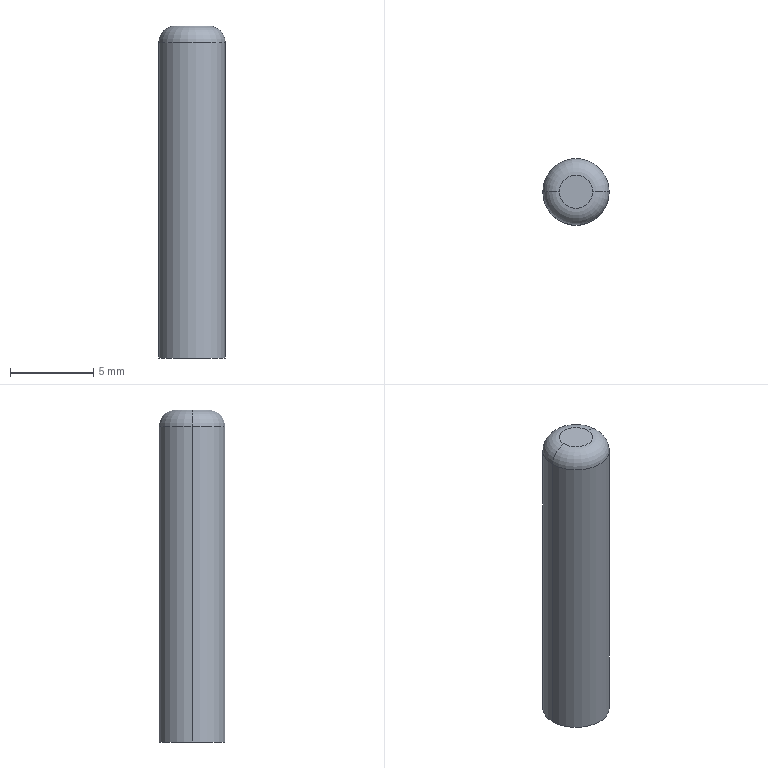Part | SolidWorks | features MirrorStock 1 | 1 solid | 10 faces | box 4 x 4 x 20 mm | volume 245.594 mm3 | cylinder 4 | torus 2 | cone 2 | plane 2 | commonest cylinder face diameters 1.6 x2 4 x2
STEP:
#1=CARTESIAN_POINT('',(11.281,-38.2,0.));
#2=VERTEX_POINT('',#1);
#3=CARTESIAN_POINT('',(9.281,-38.2,0.));
#4=VERTEX_POINT('',#3);
#5=CARTESIAN_POINT('',(10.281,-38.2,0.));
#6=DIRECTION('',(0.,0.,-1.));
#7=DIRECTION('',(1.,0.,0.));
#8=AXIS2_PLACEMENT_3D('',#5,#6,#7);
#9=CIRCLE('',#8,1.);
#10=EDGE_CURVE('',#2,#4,#9,.T.);
#11=ORIENTED_EDGE('',*,*,#10,.T.);
#12=CARTESIAN_POINT('',(8.281,-38.2,-1.));
#13=VERTEX_POINT('',#12);
#14=CARTESIAN_POINT('',(9.281,-38.2,-1.));
#15=DIRECTION('',(0.,-1.,0.));
#16=DIRECTION('',(1.,0.,0.));
#17=AXIS2_PLACEMENT_3D('',#14,#15,#16);
#18=CIRCLE('',#17,1.);
#19=EDGE_CURVE('',#4,#13,#18,.T.);
#20=ORIENTED_EDGE('',*,*,#19,.T.);
#21=CARTESIAN_POINT('',(12.281,-38.2,-1.));
#22=VERTEX_POINT('',#21);
#23=CARTESIAN_POINT('',(10.281,-38.2,-1.));
#24=DIRECTION('',(0.,0.,1.));
#25=DIRECTION('',(1.,0.,0.));
#26=AXIS2_PLACEMENT_3D('',#23,#24,#25);
#27=CIRCLE('',#26,2.);
#28=EDGE_CURVE('',#13,#22,#27,.T.);
#29=ORIENTED_EDGE('',*,*,#28,.T.);
#30=CARTESIAN_POINT('',(11.281,-38.2,-1.));
#31=DIRECTION('',(0.,1.,0.));
#32=DIRECTION('',(0.,0.,1.));
#33=AXIS2_PLACEMENT_3D('',#30,#31,#32);
#34=CIRCLE('',#33,1.);
#35=EDGE_CURVE('',#2,#22,#34,.T.);
#36=ORIENTED_EDGE('',*,*,#35,.F.);
#37=EDGE_LOOP('',(#11,#20,#29,#36));
#38=FACE_OUTER_BOUND('',#37,.T.);
#39=CARTESIAN_POINT('',(10.281,-38.2,-1.));
#40=DIRECTION('',(0.,0.,-1.));
#41=DIRECTION('',(1.,0.,0.));
#42=AXIS2_PLACEMENT_3D('',#39,#40,#41);
#43=TOROIDAL_SURFACE('',#42,1.,1.);
#44=ADVANCED_FACE('',(#38),#43,.T.);
#45=CARTESIAN_POINT('',(10.281,-39.,-18.5));
#46=VERTEX_POINT('',#45);
#47=CARTESIAN_POINT('',(10.281,-37.4,-18.5));
#48=VERTEX_POINT('',#47);
#49=CARTESIAN_POINT('',(10.281,-38.2,-18.5));
#50=DIRECTION('',(0.,0.,1.));
#51=DIRECTION('',(0.,-1.,0.));
#52=AXIS2_PLACEMENT_3D('',#49,#50,#51);
#53=CIRCLE('',#52,0.8);
#54=EDGE_CURVE('',#46,#48,#53,.T.);
#55=ORIENTED_EDGE('',*,*,#54,.T.);
#56=CARTESIAN_POINT('',(10.281,-37.4,-20.));
#57=VERTEX_POINT('',#56);
#58=CARTESIAN_POINT('',(10.281,-37.4,-23.7));
#59=DIRECTION('',(0.,0.,-1.));
#60=VECTOR('',#59,1000.);
#61=LINE('',#58,#60);
#62=EDGE_CURVE('',#48,#57,#61,.T.);
#63=ORIENTED_EDGE('',*,*,#62,.T.);
#64=CARTESIAN_POINT('',(10.281,-39.,-20.));
#65=VERTEX_POINT('',#64);
#66=CARTESIAN_POINT('',(10.281,-38.2,-20.));
#67=DIRECTION('',(0.,0.,1.));
#68=DIRECTION('',(1.,0.,0.));
#69=AXIS2_PLACEMENT_3D('',#66,#67,#68);
#70=CIRCLE('',#69,0.8);
#71=EDGE_CURVE('',#65,#57,#70,.T.);
#72=ORIENTED_EDGE('',*,*,#71,.F.);
#73=CARTESIAN_POINT('',(10.281,-39.,-23.7));
#74=DIRECTION('',(0.,0.,-1.));
#75=VECTOR('',#74,1000.);
#76=LINE('',#73,#75);
#77=EDGE_CURVE('',#46,#65,#76,.T.);
#78=ORIENTED_EDGE('',*,*,#77,.F.);
#79=EDGE_LOOP('',(#55,#63,#72,#78));
#80=FACE_OUTER_BOUND('',#79,.T.);
#81=CARTESIAN_POINT('',(10.281,-38.2,-23.7));
#82=DIRECTION('',(0.,0.,-1.));
#83=DIRECTION('',(0.,-1.,0.));
#84=AXIS2_PLACEMENT_3D('',#81,#82,#83);
#85=CYLINDRICAL_SURFACE('',#84,0.8);
#86=ADVANCED_FACE('',(#80),#85,.F.);
#87=CARTESIAN_POINT('',(10.281,-38.2,-18.019));
#88=VERTEX_POINT('',#87);
#89=CARTESIAN_POINT('',(10.281,-39.,-18.5));
#90=DIRECTION('',(0.,-0.8572,-0.515));
#91=VECTOR('',#90,1000.);
#92=LINE('',#89,#91);
#93=EDGE_CURVE('',#88,#46,#92,.T.);
#94=ORIENTED_EDGE('',*,*,#93,.F.);
#95=CARTESIAN_POINT('',(10.281,-37.4,-18.5));
#96=DIRECTION('',(0.,0.8572,-0.515));
#97=VECTOR('',#96,1000.);
#98=LINE('',#95,#97);
#99=EDGE_CURVE('',#88,#48,#98,.T.);
#100=ORIENTED_EDGE('',*,*,#99,.T.);
#101=ORIENTED_EDGE('',*,*,#54,.F.);
#102=EDGE_LOOP('',(#94,#100,#101));
#103=FACE_OUTER_BOUND('',#102,.T.);
#104=CARTESIAN_POINT('',(10.281,-38.2,-18.5));
#105=DIRECTION('',(0.,0.,-1.));
#106=DIRECTION('',(0.,-1.,0.));
#107=AXIS2_PLACEMENT_3D('',#104,#105,#106);
#108=CONICAL_SURFACE('',#107,0.8,1.03);
#109=ADVANCED_FACE('',(#103),#108,.F.);
#110=CARTESIAN_POINT('',(8.281,-38.2,-20.));
#111=VERTEX_POINT('',#110);
#112=CARTESIAN_POINT('',(12.281,-38.2,-20.));
#113=VERTEX_POINT('',#112);
#114=CARTESIAN_POINT('',(10.281,-38.2,-20.));
#115=DIRECTION('',(0.,0.,1.));
#116=DIRECTION('',(1.,0.,0.));
#117=AXIS2_PLACEMENT_3D('',#114,#115,#116);
#118=CIRCLE('',#117,2.);
#119=EDGE_CURVE('',#111,#113,#118,.T.);
#120=ORIENTED_EDGE('',*,*,#119,.T.);
#121=CARTESIAN_POINT('',(12.281,-38.2,-20.));
#122=DIRECTION('',(0.,0.,1.));
#123=VECTOR('',#122,1000.);
#124=LINE('',#121,#123);
#125=EDGE_CURVE('',#113,#22,#124,.T.);
#126=ORIENTED_EDGE('',*,*,#125,.T.);
#127=ORIENTED_EDGE('',*,*,#28,.F.);
#128=CARTESIAN_POINT('',(8.281,-38.2,-20.));
#129=DIRECTION('',(0.,0.,1.));
#130=VECTOR('',#129,1000.);
#131=LINE('',#128,#130);
#132=EDGE_CURVE('',#111,#13,#131,.T.);
#133=ORIENTED_EDGE('',*,*,#132,.F.);
#134=EDGE_LOOP('',(#120,#126,#127,#133));
#135=FACE_OUTER_BOUND('',#134,.T.);
#136=CARTESIAN_POINT('',(10.281,-38.2,-20.));
#137=DIRECTION('',(0.,0.,1.));
#138=DIRECTION('',(-1.,0.,0.));
#139=AXIS2_PLACEMENT_3D('',#136,#137,#138);
#140=CYLINDRICAL_SURFACE('',#139,2.);
#141=ADVANCED_FACE('',(#135),#140,.T.);
#142=ORIENTED_EDGE('',*,*,#125,.F.);
#143=CARTESIAN_POINT('',(10.281,-38.2,-20.));
#144=DIRECTION('',(0.,0.,1.));
#145=DIRECTION('',(1.,0.,0.));
#146=AXIS2_PLACEMENT_3D('',#143,#144,#145);
#147=CIRCLE('',#146,2.);
#148=EDGE_CURVE('',#113,#111,#147,.T.);
#149=ORIENTED_EDGE('',*,*,#148,.T.);
#150=ORIENTED_EDGE('',*,*,#132,.T.);
#151=CARTESIAN_POINT('',(10.281,-38.2,-1.));
#152=DIRECTION('',(0.,0.,1.));
#153=DIRECTION('',(1.,0.,0.));
#154=AXIS2_PLACEMENT_3D('',#151,#152,#153);
#155=CIRCLE('',#154,2.);
#156=EDGE_CURVE('',#22,#13,#155,.T.);
#157=ORIENTED_EDGE('',*,*,#156,.F.);
#158=EDGE_LOOP('',(#142,#149,#150,#157));
#159=FACE_OUTER_BOUND('',#158,.T.);
#160=CARTESIAN_POINT('',(10.281,-38.2,-20.));
#161=DIRECTION('',(0.,0.,1.));
#162=DIRECTION('',(-1.,0.,0.));
#163=AXIS2_PLACEMENT_3D('',#160,#161,#162);
#164=CYLINDRICAL_SURFACE('',#163,2.);
#165=ADVANCED_FACE('',(#159),#164,.T.);
#166=ORIENTED_EDGE('',*,*,#71,.T.);
#167=CARTESIAN_POINT('',(10.281,-38.2,-20.));
#168=DIRECTION('',(0.,0.,1.));
#169=DIRECTION('',(1.,0.,0.));
#170=AXIS2_PLACEMENT_3D('',#167,#168,#169);
#171=CIRCLE('',#170,0.8);
#172=EDGE_CURVE('',#57,#65,#171,.T.);
#173=ORIENTED_EDGE('',*,*,#172,.T.);
#174=EDGE_LOOP('',(#166,#173));
#175=FACE_BOUND('',#174,.T.);
#176=ORIENTED_EDGE('',*,*,#119,.F.);
#177=ORIENTED_EDGE('',*,*,#148,.F.);
#178=EDGE_LOOP('',(#176,#177));
#179=FACE_OUTER_BOUND('',#178,.T.);
#180=CARTESIAN_POINT('',(10.281,-38.2,-20.));
#181=DIRECTION('',(0.,0.,-1.));
#182=DIRECTION('',(1.,0.,0.));
#183=AXIS2_PLACEMENT_3D('',#180,#181,#182);
#184=PLANE('',#183);
#185=ADVANCED_FACE('',(#175,#179),#184,.T.);
#186=ORIENTED_EDGE('',*,*,#10,.F.);
#187=CARTESIAN_POINT('',(10.281,-38.2,0.));
#188=DIRECTION('',(0.,0.,-1.));
#189=DIRECTION('',(1.,0.,0.));
#190=AXIS2_PLACEMENT_3D('',#187,#188,#189);
#191=CIRCLE('',#190,1.);
#192=EDGE_CURVE('',#4,#2,#191,.T.);
#193=ORIENTED_EDGE('',*,*,#192,.F.);
#194=EDGE_LOOP('',(#186,#193));
#195=FACE_OUTER_BOUND('',#194,.T.);
#196=CARTESIAN_POINT('',(10.281,-38.2,0.));
#197=DIRECTION('',(0.,0.,-1.));
#198=DIRECTION('',(1.,0.,0.));
#199=AXIS2_PLACEMENT_3D('',#196,#197,#198);
#200=PLANE('',#199);
#201=ADVANCED_FACE('',(#195),#200,.F.);
#202=ORIENTED_EDGE('',*,*,#99,.F.);
#203=ORIENTED_EDGE('',*,*,#93,.T.);
#204=CARTESIAN_POINT('',(10.281,-38.2,-18.5));
#205=DIRECTION('',(0.,0.,1.));
#206=DIRECTION('',(0.,-1.,0.));
#207=AXIS2_PLACEMENT_3D('',#204,#205,#206);
#208=CIRCLE('',#207,0.8);
#209=EDGE_CURVE('',#48,#46,#208,.T.);
#210=ORIENTED_EDGE('',*,*,#209,.F.);
#211=EDGE_LOOP('',(#202,#203,#210));
#212=FACE_OUTER_BOUND('',#211,.T.);
#213=CARTESIAN_POINT('',(10.281,-38.2,-18.5));
#214=DIRECTION('',(0.,0.,-1.));
#215=DIRECTION('',(0.,-1.,0.));
#216=AXIS2_PLACEMENT_3D('',#213,#214,#215);
#217=CONICAL_SURFACE('',#216,0.8,1.03);
#218=ADVANCED_FACE('',(#212),#217,.F.);
#219=ORIENTED_EDGE('',*,*,#62,.F.);
#220=ORIENTED_EDGE('',*,*,#209,.T.);
#221=ORIENTED_EDGE('',*,*,#77,.T.);
#222=ORIENTED_EDGE('',*,*,#172,.F.);
#223=EDGE_LOOP('',(#219,#220,#221,#222));
#224=FACE_OUTER_BOUND('',#223,.T.);
#225=CARTESIAN_POINT('',(10.281,-38.2,-23.7));
#226=DIRECTION('',(0.,0.,-1.));
#227=DIRECTION('',(0.,-1.,0.));
#228=AXIS2_PLACEMENT_3D('',#225,#226,#227);
#229=CYLINDRICAL_SURFACE('',#228,0.8);
#230=ADVANCED_FACE('',(#224),#229,.F.);
#231=ORIENTED_EDGE('',*,*,#19,.F.);
#232=ORIENTED_EDGE('',*,*,#192,.T.);
#233=ORIENTED_EDGE('',*,*,#35,.T.);
#234=ORIENTED_EDGE('',*,*,#156,.T.);
#235=EDGE_LOOP('',(#231,#232,#233,#234));
#236=FACE_OUTER_BOUND('',#235,.T.);
#237=CARTESIAN_POINT('',(10.281,-38.2,-1.));
#238=DIRECTION('',(0.,0.,-1.));
#239=DIRECTION('',(1.,0.,0.));
#240=AXIS2_PLACEMENT_3D('',#237,#238,#239);
#241=TOROIDAL_SURFACE('',#240,1.,1.);
#242=ADVANCED_FACE('',(#236),#241,.T.);
#243=CLOSED_SHELL('',(#44,#86,#109,#141,#165,#185,#201,#218,#230,#242));
#244=MANIFOLD_SOLID_BREP('',#243);
#245=CARTESIAN_POINT('',(0.,0.,0.));
#246=DIRECTION('',(0.,0.,1.));
#247=DIRECTION('',(1.,0.,0.));
#248=AXIS2_PLACEMENT_3D('',#245,#246,#247);
#249=(LENGTH_UNIT()NAMED_UNIT(*)SI_UNIT(.MILLI.,.METRE.));
#250=UNCERTAINTY_MEASURE_WITH_UNIT(LENGTH_MEASURE(0.00001),#249,'','');
#251=(NAMED_UNIT(*)PLANE_ANGLE_UNIT()SI_UNIT($,.RADIAN.));
#252=(NAMED_UNIT(*)SI_UNIT($,.STERADIAN.)SOLID_ANGLE_UNIT());
#253=(GEOMETRIC_REPRESENTATION_CONTEXT(3)GLOBAL_UNCERTAINTY_ASSIGNED_CONTEXT((#250))GLOBAL_UNIT_ASSIGNED_CONTEXT((#249,#251,#252))REPRESENTATION_CONTEXT('',''));
#254=ADVANCED_BREP_SHAPE_REPRESENTATION('',(#244,#248),#253);